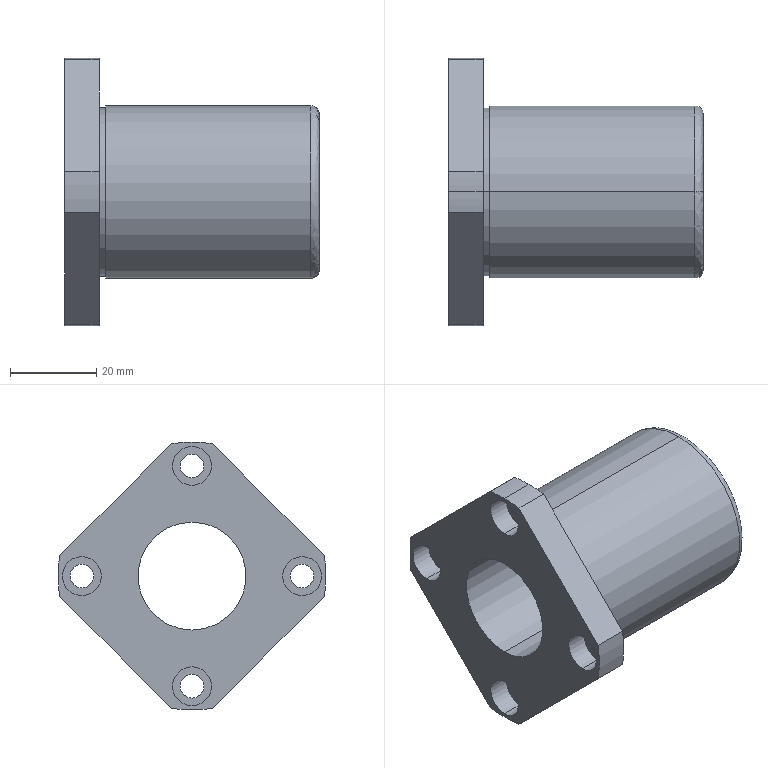Part | STEP file | LHFSF25-2.15-02-02-a_2 | 1 solid | 41 faces | box 59 x 62 x 62 mm | volume 52716 mm3 | cylinder 27 | plane 12 | spline 2 | commonest cylinder face diameters 5.5 x8 9 x8 62 x5 25 x2 39 x2 40 x2